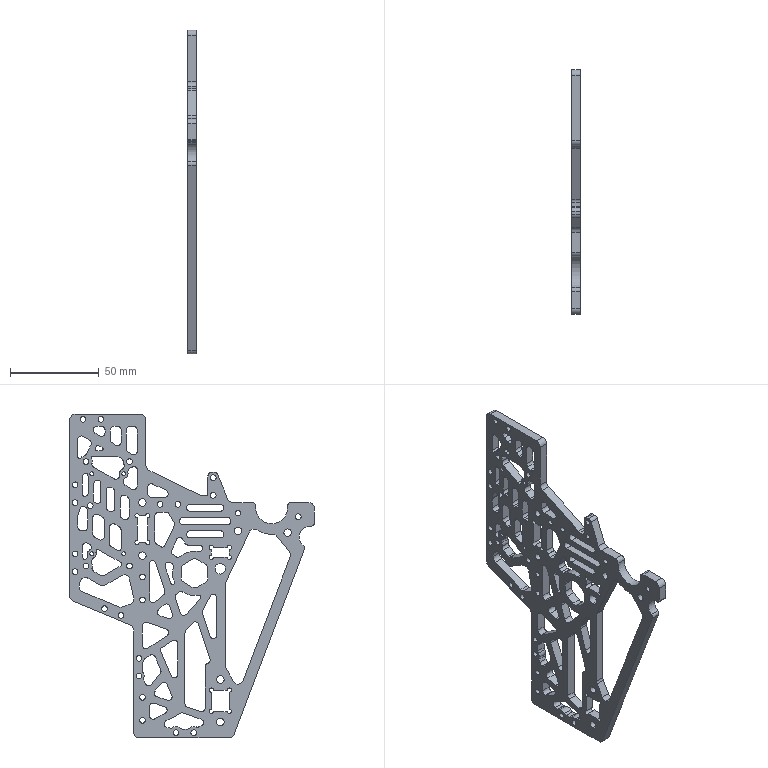Part | SolidWorks | features Fillet 3, Extrusion 1, ICE 1 | 1 solid | 507 faces | box 5 x 138 x 183 mm | volume 44741 mm3 | cylinder 343 | plane 164 | commonest cylinder face diameters 4 x177 3.2 x54 6 x34 2.4 x18 2 x13 4.2 x12